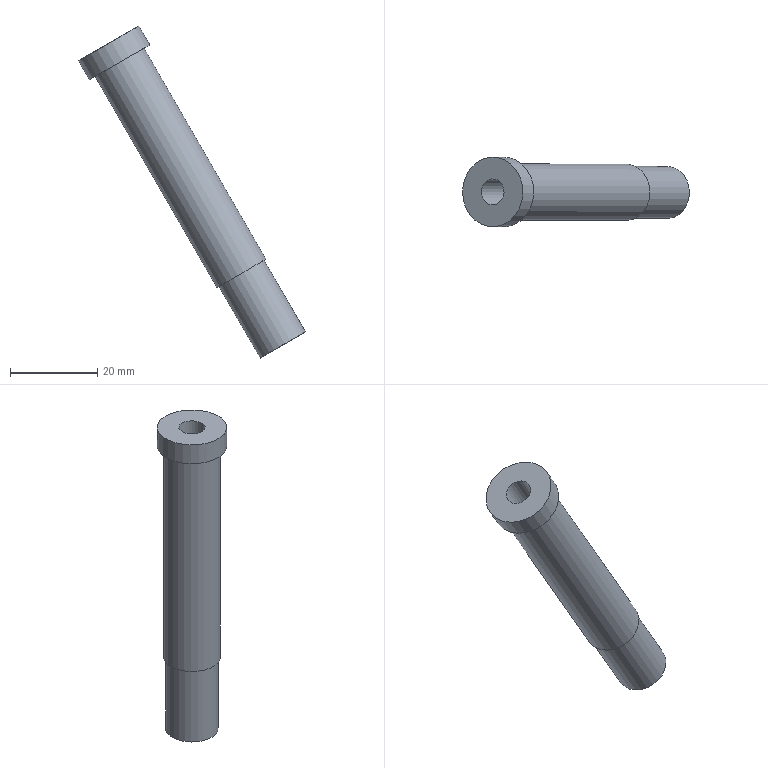Part | NX | features solid 2 | 1 solid | 9 faces | box 52.124 x 16 x 76.282 mm | volume 10203 mm3 | cylinder 4 | plane 4 | cone 1 | commonest cylinder face diameters 6 x1 12 x1 13 x1 16 x1
STEP:
#1=CARTESIAN_POINT('',(-262.415,133.822,57.303));
#2=VERTEX_POINT('',#1);
#3=CARTESIAN_POINT('',(-268.042,134.,54.054));
#4=DIRECTION('',(-0.5,0.,0.866));
#5=DIRECTION('',(0.8657,-0.02744,0.4998));
#6=AXIS2_PLACEMENT_3D('',#3,#4,#5);
#7=CIRCLE('',#6,6.5);
#8=EDGE_CURVE('',#2,#2,#7,.T.);
#9=ORIENTED_EDGE('',*,*,#8,.T.);
#10=EDGE_LOOP('',(#9));
#11=FACE_BOUND('',#10,.T.);
#12=CARTESIAN_POINT('',(-290.415,133.822,105.801));
#13=VERTEX_POINT('',#12);
#14=CARTESIAN_POINT('',(-296.042,134.,102.552));
#15=DIRECTION('',(-0.5,0.,0.866));
#16=DIRECTION('',(0.8657,-0.02744,0.4998));
#17=AXIS2_PLACEMENT_3D('',#14,#15,#16);
#18=CIRCLE('',#17,6.5);
#19=EDGE_CURVE('',#13,#13,#18,.T.);
#20=ORIENTED_EDGE('',*,*,#19,.F.);
#21=EDGE_LOOP('',(#20));
#22=FACE_BOUND('',#21,.T.);
#23=CARTESIAN_POINT('',(-298.542,134.,106.882));
#24=DIRECTION('',(0.5,0.,-0.866));
#25=DIRECTION('',(-0.8657,0.02744,-0.4998));
#26=AXIS2_PLACEMENT_3D('',#23,#24,#25);
#27=CYLINDRICAL_SURFACE('',#26,6.5);
#28=ADVANCED_FACE('',(#11,#22),#27,.T.);
#29=CARTESIAN_POINT('',(-262.848,133.835,57.053));
#30=VERTEX_POINT('',#29);
#31=CARTESIAN_POINT('',(-268.042,134.,54.054));
#32=DIRECTION('',(-0.5,0.,0.866));
#33=DIRECTION('',(0.8657,-0.02744,0.4998));
#34=AXIS2_PLACEMENT_3D('',#31,#32,#33);
#35=CIRCLE('',#34,6.);
#36=EDGE_CURVE('',#30,#30,#35,.T.);
#37=ORIENTED_EDGE('',*,*,#36,.T.);
#38=EDGE_LOOP('',(#37));
#39=FACE_BOUND('',#38,.T.);
#40=ORIENTED_EDGE('',*,*,#8,.F.);
#41=EDGE_LOOP('',(#40));
#42=FACE_BOUND('',#41,.T.);
#43=CARTESIAN_POINT('',(-268.042,134.,54.054));
#44=DIRECTION('',(-0.5,0.,0.866));
#45=DIRECTION('',(0.8657,-0.02744,0.4998));
#46=AXIS2_PLACEMENT_3D('',#43,#44,#45);
#47=PLANE('',#46);
#48=ADVANCED_FACE('',(#39,#42),#47,.F.);
#49=CARTESIAN_POINT('',(-289.117,133.781,106.55));
#50=VERTEX_POINT('',#49);
#51=CARTESIAN_POINT('',(-296.042,134.,102.552));
#52=DIRECTION('',(-0.5,0.,0.866));
#53=DIRECTION('',(0.8657,-0.02744,0.4998));
#54=AXIS2_PLACEMENT_3D('',#51,#52,#53);
#55=CIRCLE('',#54,8.);
#56=EDGE_CURVE('',#50,#50,#55,.T.);
#57=ORIENTED_EDGE('',*,*,#56,.F.);
#58=EDGE_LOOP('',(#57));
#59=FACE_BOUND('',#58,.T.);
#60=ORIENTED_EDGE('',*,*,#19,.T.);
#61=EDGE_LOOP('',(#60));
#62=FACE_BOUND('',#61,.T.);
#63=CARTESIAN_POINT('',(-296.042,134.,102.552));
#64=DIRECTION('',(-0.5,0.,0.866));
#65=DIRECTION('',(0.8657,-0.02744,0.4998));
#66=AXIS2_PLACEMENT_3D('',#63,#64,#65);
#67=PLANE('',#66);
#68=ADVANCED_FACE('',(#59,#62),#67,.F.);
#69=ORIENTED_EDGE('',*,*,#56,.T.);
#70=EDGE_LOOP('',(#69));
#71=FACE_BOUND('',#70,.T.);
#72=CARTESIAN_POINT('',(-291.617,133.781,110.881));
#73=VERTEX_POINT('',#72);
#74=CARTESIAN_POINT('',(-298.542,134.,106.882));
#75=DIRECTION('',(-0.5,0.,0.866));
#76=DIRECTION('',(0.8657,-0.02744,0.4998));
#77=AXIS2_PLACEMENT_3D('',#74,#75,#76);
#78=CIRCLE('',#77,8.);
#79=EDGE_CURVE('',#73,#73,#78,.T.);
#80=ORIENTED_EDGE('',*,*,#79,.F.);
#81=EDGE_LOOP('',(#80));
#82=FACE_BOUND('',#81,.T.);
#83=CARTESIAN_POINT('',(-296.042,134.,102.552));
#84=DIRECTION('',(-0.5,0.,0.866));
#85=DIRECTION('',(0.8657,-0.02744,0.4998));
#86=AXIS2_PLACEMENT_3D('',#83,#84,#85);
#87=CYLINDRICAL_SURFACE('',#86,8.);
#88=ADVANCED_FACE('',(#71,#82),#87,.T.);
#89=CARTESIAN_POINT('',(-301.14,134.082,105.383));
#90=VERTEX_POINT('',#89);
#91=CARTESIAN_POINT('',(-298.542,134.,106.882));
#92=DIRECTION('',(0.5,0.,-0.866));
#93=DIRECTION('',(-0.8657,0.02744,-0.4998));
#94=AXIS2_PLACEMENT_3D('',#91,#92,#93);
#95=CIRCLE('',#94,3.);
#96=EDGE_CURVE('',#90,#90,#95,.T.);
#97=ORIENTED_EDGE('',*,*,#96,.T.);
#98=EDGE_LOOP('',(#97));
#99=FACE_BOUND('',#98,.T.);
#100=ORIENTED_EDGE('',*,*,#79,.T.);
#101=EDGE_LOOP('',(#100));
#102=FACE_BOUND('',#101,.T.);
#103=CARTESIAN_POINT('',(-298.542,134.,106.882));
#104=DIRECTION('',(-0.5,0.,0.866));
#105=DIRECTION('',(0.8657,-0.02744,0.4998));
#106=AXIS2_PLACEMENT_3D('',#103,#104,#105);
#107=PLANE('',#106);
#108=ADVANCED_FACE('',(#99,#102),#107,.T.);
#109=CARTESIAN_POINT('',(-253.348,133.835,40.599));
#110=VERTEX_POINT('',#109);
#111=CARTESIAN_POINT('',(-258.542,134.,37.6));
#112=DIRECTION('',(-0.5,0.,0.866));
#113=DIRECTION('',(0.8657,-0.02744,0.4998));
#114=AXIS2_PLACEMENT_3D('',#111,#112,#113);
#115=CIRCLE('',#114,6.);
#116=EDGE_CURVE('',#110,#110,#115,.T.);
#117=ORIENTED_EDGE('',*,*,#116,.T.);
#118=EDGE_LOOP('',(#117));
#119=FACE_BOUND('',#118,.T.);
#120=ORIENTED_EDGE('',*,*,#36,.F.);
#121=EDGE_LOOP('',(#120));
#122=FACE_BOUND('',#121,.T.);
#123=CARTESIAN_POINT('',(-258.542,134.,37.6));
#124=DIRECTION('',(-0.5,0.,0.866));
#125=DIRECTION('',(0.8657,-0.02744,0.4998));
#126=AXIS2_PLACEMENT_3D('',#123,#124,#125);
#127=CYLINDRICAL_SURFACE('',#126,6.);
#128=ADVANCED_FACE('',(#119,#122),#127,.T.);
#129=ORIENTED_EDGE('',*,*,#116,.F.);
#130=EDGE_LOOP('',(#129));
#131=FACE_BOUND('',#130,.T.);
#132=CARTESIAN_POINT('',(-258.542,134.,37.6));
#133=DIRECTION('',(-0.5,0.,0.866));
#134=DIRECTION('',(0.8657,-0.02744,0.4998));
#135=AXIS2_PLACEMENT_3D('',#132,#133,#134);
#136=PLANE('',#135);
#137=ADVANCED_FACE('',(#131),#136,.F.);
#138=CARTESIAN_POINT('',(-294.64,134.082,94.124));
#139=VERTEX_POINT('',#138);
#140=CARTESIAN_POINT('',(-292.042,134.,95.624));
#141=DIRECTION('',(0.5,0.,-0.866));
#142=DIRECTION('',(-0.8657,0.02744,-0.4998));
#143=AXIS2_PLACEMENT_3D('',#140,#141,#142);
#144=CIRCLE('',#143,3.);
#145=EDGE_CURVE('',#139,#139,#144,.T.);
#146=ORIENTED_EDGE('',*,*,#145,.F.);
#147=EDGE_LOOP('',(#146));
#148=FACE_BOUND('',#147,.T.);
#149=CARTESIAN_POINT('',(-291.176,134.,94.124));
#150=VERTEX_POINT('',#149);
#151=VERTEX_LOOP('',#150);
#152=FACE_BOUND('',#151,.T.);
#153=CARTESIAN_POINT('',(-292.042,134.,95.624));
#154=DIRECTION('',(-0.5,0.,0.866));
#155=DIRECTION('',(0.8657,-0.02744,0.4998));
#156=AXIS2_PLACEMENT_3D('',#153,#154,#155);
#157=CONICAL_SURFACE('',#156,3.,1.047);
#158=ADVANCED_FACE('',(#148,#152),#157,.F.);
#159=ORIENTED_EDGE('',*,*,#145,.T.);
#160=EDGE_LOOP('',(#159));
#161=FACE_BOUND('',#160,.T.);
#162=ORIENTED_EDGE('',*,*,#96,.F.);
#163=EDGE_LOOP('',(#162));
#164=FACE_BOUND('',#163,.T.);
#165=CARTESIAN_POINT('',(-298.542,134.,106.882));
#166=DIRECTION('',(0.5,0.,-0.866));
#167=DIRECTION('',(-0.8657,0.02744,-0.4998));
#168=AXIS2_PLACEMENT_3D('',#165,#166,#167);
#169=CYLINDRICAL_SURFACE('',#168,3.);
#170=ADVANCED_FACE('',(#161,#164),#169,.F.);
#171=CLOSED_SHELL('',(#28,#48,#68,#88,#108,#128,#137,#158,#170));
#172=MANIFOLD_SOLID_BREP('',#171);
#173=(LENGTH_UNIT()NAMED_UNIT(*)SI_UNIT(.MILLI.,.METRE.));
#174=UNCERTAINTY_MEASURE_WITH_UNIT(LENGTH_MEASURE(0.00001),#173,'','');
#175=(NAMED_UNIT(*)PLANE_ANGLE_UNIT()SI_UNIT($,.RADIAN.));
#176=(NAMED_UNIT(*)SI_UNIT($,.STERADIAN.)SOLID_ANGLE_UNIT());
#177=(GEOMETRIC_REPRESENTATION_CONTEXT(3)GLOBAL_UNCERTAINTY_ASSIGNED_CONTEXT((#174))GLOBAL_UNIT_ASSIGNED_CONTEXT((#173,#175,#176))REPRESENTATION_CONTEXT('',''));
#178=ADVANCED_BREP_SHAPE_REPRESENTATION('',(#172),#177);